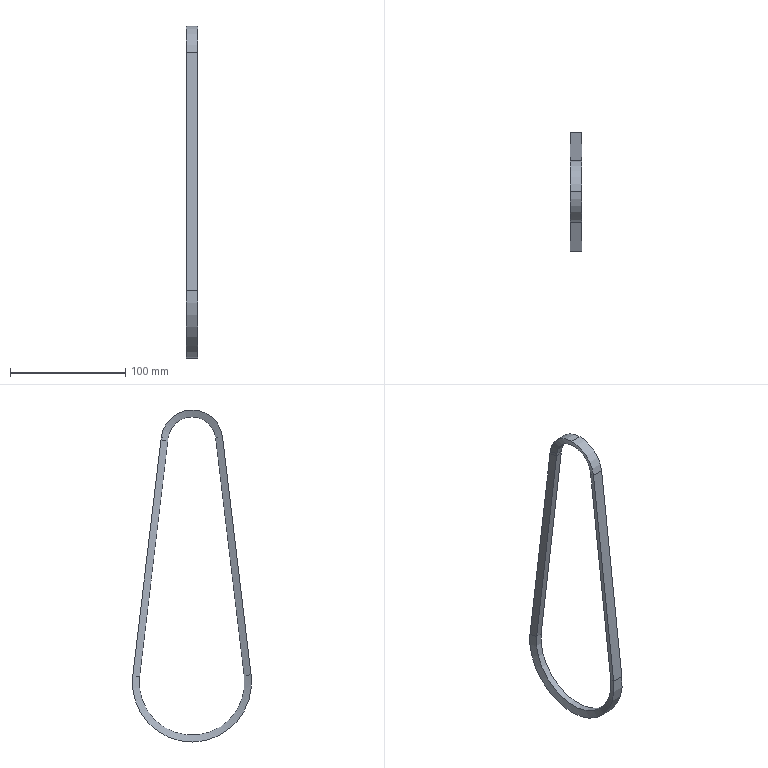Part | SolidWorks | features Sweep 1 | 1 solid | 22 faces | box 10 x 103.625 x 288.63 mm | volume 30426 mm3 | plane 12 | cylinder 6 | spline 4 | commonest cylinder face diameters 41.701 x2 53.634 x2 91.701 x1 103.625 x1
STEP:
#1=CARTESIAN_POINT('',(5.,-47.534,3.883));
#2=VERTEX_POINT('',#1);
#3=CARTESIAN_POINT('',(5.,-21.,26.817));
#4=VERTEX_POINT('',#3);
#5=CARTESIAN_POINT('',(5.,-21.,0.));
#6=DIRECTION('',(-1.,0.,0.));
#7=DIRECTION('',(0.,-0.9895,0.1448));
#8=AXIS2_PLACEMENT_3D('',#5,#6,#7);
#9=CIRCLE('',#8,26.817);
#10=EDGE_CURVE('',#2,#4,#9,.T.);
#11=ORIENTED_EDGE('',*,*,#10,.T.);
#12=CARTESIAN_POINT('',(-5.,-21.,26.817));
#13=VERTEX_POINT('',#12);
#14=CARTESIAN_POINT('',(0.,-21.,26.817));
#15=DIRECTION('',(-1.,0.,0.));
#16=VECTOR('',#15,1000.);
#17=LINE('',#14,#16);
#18=EDGE_CURVE('',#4,#13,#17,.T.);
#19=ORIENTED_EDGE('',*,*,#18,.T.);
#20=CARTESIAN_POINT('',(-5.,-47.534,3.883));
#21=VERTEX_POINT('',#20);
#22=CARTESIAN_POINT('',(-5.,-21.,0.));
#23=DIRECTION('',(-1.,0.,0.));
#24=DIRECTION('',(0.,-0.9895,0.1448));
#25=AXIS2_PLACEMENT_3D('',#22,#23,#24);
#26=CIRCLE('',#25,26.817);
#27=EDGE_CURVE('',#21,#13,#26,.T.);
#28=ORIENTED_EDGE('',*,*,#27,.F.);
#29=CARTESIAN_POINT('',(-5.,-47.534,3.883));
#30=DIRECTION('',(-1.,0.,0.));
#31=VECTOR('',#30,1000.);
#32=LINE('',#29,#31);
#33=EDGE_CURVE('',#2,#21,#32,.T.);
#34=ORIENTED_EDGE('',*,*,#33,.F.);
#35=EDGE_LOOP('',(#11,#19,#28,#34));
#36=FACE_OUTER_BOUND('',#35,.T.);
#37=CARTESIAN_POINT('',(0.,-21.,0.));
#38=DIRECTION('',(-1.,0.,0.));
#39=DIRECTION('',(0.,0.,1.));
#40=AXIS2_PLACEMENT_3D('',#37,#38,#39);
#41=CYLINDRICAL_SURFACE('',#40,26.817);
#42=ADVANCED_FACE('',(#36),#41,.T.);
#43=CARTESIAN_POINT('',(2.816,-21.,20.851));
#44=VERTEX_POINT('',#43);
#45=CARTESIAN_POINT('',(2.816,-0.2998,2.5));
#46=VERTEX_POINT('',#45);
#47=CARTESIAN_POINT('',(2.816,-21.,0.));
#48=DIRECTION('',(-1.,0.,0.));
#49=DIRECTION('',(0.,-0.993,0.1182));
#50=AXIS2_PLACEMENT_3D('',#47,#48,#49);
#51=CIRCLE('',#50,20.851);
#52=EDGE_CURVE('',#44,#46,#51,.T.);
#53=ORIENTED_EDGE('',*,*,#52,.F.);
#54=CARTESIAN_POINT('',(-2.816,-21.,20.851));
#55=VERTEX_POINT('',#54);
#56=CARTESIAN_POINT('',(0.,-21.,20.851));
#57=DIRECTION('',(-1.,0.,0.));
#58=VECTOR('',#57,1000.);
#59=LINE('',#56,#58);
#60=EDGE_CURVE('',#44,#55,#59,.T.);
#61=ORIENTED_EDGE('',*,*,#60,.T.);
#62=CARTESIAN_POINT('',(-2.816,-0.2998,2.5));
#63=VERTEX_POINT('',#62);
#64=CARTESIAN_POINT('',(-2.816,-21.,0.));
#65=DIRECTION('',(-1.,0.,0.));
#66=DIRECTION('',(0.,-0.993,0.1182));
#67=AXIS2_PLACEMENT_3D('',#64,#65,#66);
#68=CIRCLE('',#67,20.851);
#69=EDGE_CURVE('',#55,#63,#68,.T.);
#70=ORIENTED_EDGE('',*,*,#69,.T.);
#71=CARTESIAN_POINT('',(-2.816,-0.2998,2.5));
#72=DIRECTION('',(1.,0.,0.));
#73=VECTOR('',#72,1000.);
#74=LINE('',#71,#73);
#75=EDGE_CURVE('',#63,#46,#74,.T.);
#76=ORIENTED_EDGE('',*,*,#75,.T.);
#77=EDGE_LOOP('',(#53,#61,#70,#76));
#78=FACE_OUTER_BOUND('',#77,.T.);
#79=CARTESIAN_POINT('',(0.,-21.,0.));
#80=DIRECTION('',(-1.,0.,0.));
#81=DIRECTION('',(0.,0.,1.));
#82=AXIS2_PLACEMENT_3D('',#79,#80,#81);
#83=CYLINDRICAL_SURFACE('',#82,20.851);
#84=ADVANCED_FACE('',(#78),#83,.F.);
#85=CARTESIAN_POINT('',(-5.,5.7,2.5));
#86=VERTEX_POINT('',#85);
#87=CARTESIAN_POINT('',(-5.,5.7,2.5));
#88=DIRECTION('',(0.342,-0.9397,0.));
#89=VECTOR('',#88,1000.);
#90=LINE('',#87,#89);
#91=EDGE_CURVE('',#86,#63,#90,.T.);
#92=ORIENTED_EDGE('',*,*,#91,.F.);
#93=CARTESIAN_POINT('',(-5.,6.,0.));
#94=VERTEX_POINT('',#93);
#95=CARTESIAN_POINT('',(-5.,5.7,2.5));
#96=DIRECTION('',(0.,0.119,-0.9929));
#97=VECTOR('',#96,1000.);
#98=LINE('',#95,#97);
#99=EDGE_CURVE('',#86,#94,#98,.T.);
#100=ORIENTED_EDGE('',*,*,#99,.T.);
#101=CARTESIAN_POINT('',(-2.816,0.,0.));
#102=VERTEX_POINT('',#101);
#103=CARTESIAN_POINT('',(-5.,6.,0.));
#104=DIRECTION('',(0.342,-0.9397,0.));
#105=VECTOR('',#104,1000.);
#106=LINE('',#103,#105);
#107=EDGE_CURVE('',#94,#102,#106,.T.);
#108=ORIENTED_EDGE('',*,*,#107,.T.);
#109=CARTESIAN_POINT('',(-2.816,-0.2998,2.5));
#110=DIRECTION('',(0.,0.119,-0.9929));
#111=VECTOR('',#110,1000.);
#112=LINE('',#109,#111);
#113=EDGE_CURVE('',#63,#102,#112,.T.);
#114=ORIENTED_EDGE('',*,*,#113,.F.);
#115=EDGE_LOOP('',(#92,#100,#108,#114));
#116=FACE_OUTER_BOUND('',#115,.T.);
#117=CARTESIAN_POINT('',(-5.,5.7,2.5));
#118=DIRECTION('',(0.9389,0.3417,0.04097));
#119=DIRECTION('',(-0.342,0.9397,0.));
#120=AXIS2_PLACEMENT_3D('',#117,#118,#119);
#121=PLANE('',#120);
#122=ADVANCED_FACE('',(#116),#121,.F.);
#123=CARTESIAN_POINT('',(-2.816,24.522,-204.524));
#124=VERTEX_POINT('',#123);
#125=CARTESIAN_POINT('',(-2.816,0.,0.));
#126=DIRECTION('',(0.,0.119,-0.9929));
#127=VECTOR('',#126,1000.);
#128=LINE('',#125,#127);
#129=EDGE_CURVE('',#102,#124,#128,.T.);
#130=ORIENTED_EDGE('',*,*,#129,.F.);
#131=ORIENTED_EDGE('',*,*,#107,.F.);
#132=CARTESIAN_POINT('',(-5.,30.522,-204.524));
#133=VERTEX_POINT('',#132);
#134=CARTESIAN_POINT('',(-5.,6.,0.));
#135=DIRECTION('',(0.,0.119,-0.9929));
#136=VECTOR('',#135,1000.);
#137=LINE('',#134,#136);
#138=EDGE_CURVE('',#94,#133,#137,.T.);
#139=ORIENTED_EDGE('',*,*,#138,.T.);
#140=CARTESIAN_POINT('',(-5.,30.522,-204.524));
#141=DIRECTION('',(0.342,-0.9397,0.));
#142=VECTOR('',#141,1000.);
#143=LINE('',#140,#142);
#144=EDGE_CURVE('',#133,#124,#143,.T.);
#145=ORIENTED_EDGE('',*,*,#144,.T.);
#146=EDGE_LOOP('',(#130,#131,#139,#145));
#147=FACE_OUTER_BOUND('',#146,.T.);
#148=CARTESIAN_POINT('',(-5.,6.,0.));
#149=DIRECTION('',(0.9389,0.3417,0.04097));
#150=DIRECTION('',(-0.342,0.9397,0.));
#151=AXIS2_PLACEMENT_3D('',#148,#149,#150);
#152=PLANE('',#151);
#153=ADVANCED_FACE('',(#147),#152,.F.);
#154=CARTESIAN_POINT('',(2.816,0.,0.));
#155=VERTEX_POINT('',#154);
#156=CARTESIAN_POINT('',(2.816,24.522,-204.524));
#157=VERTEX_POINT('',#156);
#158=CARTESIAN_POINT('',(2.816,0.,0.));
#159=DIRECTION('',(0.,0.119,-0.9929));
#160=VECTOR('',#159,1000.);
#161=LINE('',#158,#160);
#162=EDGE_CURVE('',#155,#157,#161,.T.);
#163=ORIENTED_EDGE('',*,*,#162,.F.);
#164=CARTESIAN_POINT('',(-2.816,0.,0.));
#165=DIRECTION('',(1.,0.,0.));
#166=VECTOR('',#165,1000.);
#167=LINE('',#164,#166);
#168=EDGE_CURVE('',#102,#155,#167,.T.);
#169=ORIENTED_EDGE('',*,*,#168,.F.);
#170=ORIENTED_EDGE('',*,*,#129,.T.);
#171=CARTESIAN_POINT('',(-2.816,24.522,-204.524));
#172=DIRECTION('',(1.,0.,0.));
#173=VECTOR('',#172,1000.);
#174=LINE('',#171,#173);
#175=EDGE_CURVE('',#124,#157,#174,.T.);
#176=ORIENTED_EDGE('',*,*,#175,.T.);
#177=EDGE_LOOP('',(#163,#169,#170,#176));
#178=FACE_OUTER_BOUND('',#177,.T.);
#179=CARTESIAN_POINT('',(-2.816,0.,0.));
#180=DIRECTION('',(0.,0.9929,0.119));
#181=DIRECTION('',(0.,-0.119,0.9929));
#182=AXIS2_PLACEMENT_3D('',#179,#180,#181);
#183=PLANE('',#182);
#184=ADVANCED_FACE('',(#178),#183,.F.);
#185=CARTESIAN_POINT('',(5.,6.,0.));
#186=VERTEX_POINT('',#185);
#187=CARTESIAN_POINT('',(5.,30.522,-204.524));
#188=VERTEX_POINT('',#187);
#189=CARTESIAN_POINT('',(5.,6.,0.));
#190=DIRECTION('',(0.,0.119,-0.9929));
#191=VECTOR('',#190,1000.);
#192=LINE('',#189,#191);
#193=EDGE_CURVE('',#186,#188,#192,.T.);
#194=ORIENTED_EDGE('',*,*,#193,.F.);
#195=CARTESIAN_POINT('',(5.,6.,0.));
#196=DIRECTION('',(0.342,0.9397,0.));
#197=VECTOR('',#196,1000.);
#198=LINE('',#195,#197);
#199=EDGE_CURVE('',#155,#186,#198,.T.);
#200=ORIENTED_EDGE('',*,*,#199,.F.);
#201=ORIENTED_EDGE('',*,*,#162,.T.);
#202=CARTESIAN_POINT('',(5.,30.522,-204.524));
#203=DIRECTION('',(0.342,0.9397,0.));
#204=VECTOR('',#203,1000.);
#205=LINE('',#202,#204);
#206=EDGE_CURVE('',#157,#188,#205,.T.);
#207=ORIENTED_EDGE('',*,*,#206,.T.);
#208=EDGE_LOOP('',(#194,#200,#201,#207));
#209=FACE_OUTER_BOUND('',#208,.T.);
#210=CARTESIAN_POINT('',(5.,6.,0.));
#211=DIRECTION('',(-0.9389,0.3417,0.04097));
#212=DIRECTION('',(-0.342,-0.9397,0.));
#213=AXIS2_PLACEMENT_3D('',#210,#211,#212);
#214=PLANE('',#213);
#215=ADVANCED_FACE('',(#209),#214,.F.);
#216=CARTESIAN_POINT('',(-5.,30.522,-204.524));
#217=DIRECTION('',(-1.,0.,0.));
#218=VECTOR('',#217,1000.);
#219=LINE('',#216,#218);
#220=EDGE_CURVE('',#188,#133,#219,.T.);
#221=ORIENTED_EDGE('',*,*,#220,.T.);
#222=ORIENTED_EDGE('',*,*,#138,.F.);
#223=CARTESIAN_POINT('',(-5.,6.,0.));
#224=DIRECTION('',(-1.,0.,0.));
#225=VECTOR('',#224,1000.);
#226=LINE('',#223,#225);
#227=EDGE_CURVE('',#186,#94,#226,.T.);
#228=ORIENTED_EDGE('',*,*,#227,.F.);
#229=ORIENTED_EDGE('',*,*,#193,.T.);
#230=EDGE_LOOP('',(#221,#222,#228,#229));
#231=FACE_OUTER_BOUND('',#230,.T.);
#232=CARTESIAN_POINT('',(-5.,6.,0.));
#233=DIRECTION('',(0.,-0.9929,-0.119));
#234=DIRECTION('',(0.,0.119,-0.9929));
#235=AXIS2_PLACEMENT_3D('',#232,#233,#234);
#236=PLANE('',#235);
#237=ADVANCED_FACE('',(#231),#236,.F.);
#238=CARTESIAN_POINT('',(-2.816,-66.527,-204.559));
#239=VERTEX_POINT('',#238);
#240=CARTESIAN_POINT('',(-2.816,-21.,-210.));
#241=DIRECTION('',(-1.,0.,0.));
#242=DIRECTION('',(0.,0.9928,0.1194));
#243=AXIS2_PLACEMENT_3D('',#240,#241,#242);
#244=CIRCLE('',#243,45.851);
#245=EDGE_CURVE('',#124,#239,#244,.T.);
#246=ORIENTED_EDGE('',*,*,#245,.F.);
#247=ORIENTED_EDGE('',*,*,#144,.F.);
#248=CARTESIAN_POINT('',(-5.,-72.357,-203.141));
#249=VERTEX_POINT('',#248);
#250=CARTESIAN_POINT('',(-5.,-21.,-210.));
#251=DIRECTION('',(-1.,0.,0.));
#252=DIRECTION('',(0.,0.9944,0.1057));
#253=AXIS2_PLACEMENT_3D('',#250,#251,#252);
#254=CIRCLE('',#253,51.813);
#255=EDGE_CURVE('',#133,#249,#254,.T.);
#256=ORIENTED_EDGE('',*,*,#255,.T.);
#257=CARTESIAN_POINT('',(-5.,-72.357,-203.141));
#258=DIRECTION('',(0.342,0.9131,-0.2221));
#259=VECTOR('',#258,1000.);
#260=LINE('',#257,#259);
#261=EDGE_CURVE('',#249,#239,#260,.T.);
#262=ORIENTED_EDGE('',*,*,#261,.T.);
#263=EDGE_LOOP('',(#246,#247,#256,#262));
#264=FACE_OUTER_BOUND('',#263,.T.);
#265=CARTESIAN_POINT('',(-5.,30.522,-204.524));
#266=CARTESIAN_POINT('',(-5.,34.043,-237.642));
#267=CARTESIAN_POINT('',(-5.,11.606,-262.256));
#268=CARTESIAN_POINT('',(-5.,-21.696,-261.808));
#269=CARTESIAN_POINT('',(-5.,-54.998,-261.36));
#270=CARTESIAN_POINT('',(-5.,-76.766,-236.153));
#271=CARTESIAN_POINT('',(-5.,-72.357,-203.141));
#272=CARTESIAN_POINT('',(-2.816,24.522,-204.524));
#273=CARTESIAN_POINT('',(-2.816,28.043,-233.786));
#274=CARTESIAN_POINT('',(-2.816,8.491,-255.839));
#275=CARTESIAN_POINT('',(-2.816,-20.982,-255.851));
#276=CARTESIAN_POINT('',(-2.816,-50.455,-255.862));
#277=CARTESIAN_POINT('',(-2.816,-70.024,-233.824));
#278=CARTESIAN_POINT('',(-2.816,-66.527,-204.559));
#279=(BOUNDED_SURFACE()B_SPLINE_SURFACE(1,3,((#265,#266,#267,#268,#269,#270,#271),(#272,#273,#274,#275,#276,#277,#278)),.UNSPECIFIED.,.F.,.F.,.T.)B_SPLINE_SURFACE_WITH_KNOTS((2,2),(4,3,4),(0.,1.),(0.,0.5,1.),.UNSPECIFIED.)GEOMETRIC_REPRESENTATION_ITEM()RATIONAL_B_SPLINE_SURFACE(((1.,0.7758,0.7758,1.,0.7758,0.7758,1.),(1.,0.7758,0.7758,1.,0.7758,0.7758,1.)))REPRESENTATION_ITEM('')SURFACE());
#280=ADVANCED_FACE('',(#264),#279,.F.);
#281=CARTESIAN_POINT('',(2.816,-66.527,-204.559));
#282=VERTEX_POINT('',#281);
#283=CARTESIAN_POINT('',(2.816,-21.,-210.));
#284=DIRECTION('',(-1.,0.,0.));
#285=DIRECTION('',(0.,0.9928,0.1194));
#286=AXIS2_PLACEMENT_3D('',#283,#284,#285);
#287=CIRCLE('',#286,45.851);
#288=EDGE_CURVE('',#157,#282,#287,.T.);
#289=ORIENTED_EDGE('',*,*,#288,.F.);
#290=ORIENTED_EDGE('',*,*,#175,.F.);
#291=ORIENTED_EDGE('',*,*,#245,.T.);
#292=CARTESIAN_POINT('',(-2.816,-66.527,-204.559));
#293=DIRECTION('',(1.,0.,0.));
#294=VECTOR('',#293,1000.);
#295=LINE('',#292,#294);
#296=EDGE_CURVE('',#239,#282,#295,.T.);
#297=ORIENTED_EDGE('',*,*,#296,.T.);
#298=EDGE_LOOP('',(#289,#290,#291,#297));
#299=FACE_OUTER_BOUND('',#298,.T.);
#300=CARTESIAN_POINT('',(0.,-21.,-210.));
#301=DIRECTION('',(-1.,0.,0.));
#302=DIRECTION('',(0.,0.,1.));
#303=AXIS2_PLACEMENT_3D('',#300,#301,#302);
#304=CYLINDRICAL_SURFACE('',#303,45.851);
#305=ADVANCED_FACE('',(#299),#304,.F.);
#306=CARTESIAN_POINT('',(5.,-72.357,-203.141));
#307=VERTEX_POINT('',#306);
#308=CARTESIAN_POINT('',(5.,-21.,-210.));
#309=DIRECTION('',(-1.,0.,0.));
#310=DIRECTION('',(0.,0.9944,0.1057));
#311=AXIS2_PLACEMENT_3D('',#308,#309,#310);
#312=CIRCLE('',#311,51.813);
#313=EDGE_CURVE('',#188,#307,#312,.T.);
#314=ORIENTED_EDGE('',*,*,#313,.F.);
#315=ORIENTED_EDGE('',*,*,#206,.F.);
#316=ORIENTED_EDGE('',*,*,#288,.T.);
#317=CARTESIAN_POINT('',(5.,-72.357,-203.141));
#318=DIRECTION('',(0.342,-0.9131,0.2221));
#319=VECTOR('',#318,1000.);
#320=LINE('',#317,#319);
#321=EDGE_CURVE('',#282,#307,#320,.T.);
#322=ORIENTED_EDGE('',*,*,#321,.T.);
#323=EDGE_LOOP('',(#314,#315,#316,#322));
#324=FACE_OUTER_BOUND('',#323,.T.);
#325=CARTESIAN_POINT('',(2.816,24.522,-204.524));
#326=CARTESIAN_POINT('',(2.816,28.043,-233.786));
#327=CARTESIAN_POINT('',(2.816,8.491,-255.839));
#328=CARTESIAN_POINT('',(2.816,-20.982,-255.851));
#329=CARTESIAN_POINT('',(2.816,-50.455,-255.862));
#330=CARTESIAN_POINT('',(2.816,-70.024,-233.824));
#331=CARTESIAN_POINT('',(2.816,-66.527,-204.559));
#332=CARTESIAN_POINT('',(5.,30.522,-204.524));
#333=CARTESIAN_POINT('',(5.,34.043,-237.642));
#334=CARTESIAN_POINT('',(5.,11.606,-262.256));
#335=CARTESIAN_POINT('',(5.,-21.696,-261.808));
#336=CARTESIAN_POINT('',(5.,-54.998,-261.36));
#337=CARTESIAN_POINT('',(5.,-76.766,-236.153));
#338=CARTESIAN_POINT('',(5.,-72.357,-203.141));
#339=(BOUNDED_SURFACE()B_SPLINE_SURFACE(1,3,((#325,#326,#327,#328,#329,#330,#331),(#332,#333,#334,#335,#336,#337,#338)),.UNSPECIFIED.,.F.,.F.,.T.)B_SPLINE_SURFACE_WITH_KNOTS((2,2),(4,3,4),(0.,1.),(0.,0.5,1.),.UNSPECIFIED.)GEOMETRIC_REPRESENTATION_ITEM()RATIONAL_B_SPLINE_SURFACE(((1.,0.7758,0.7758,1.,0.7758,0.7758,1.),(1.,0.7758,0.7758,1.,0.7758,0.7758,1.)))REPRESENTATION_ITEM('')SURFACE());
#340=ADVANCED_FACE('',(#324),#339,.F.);
#341=CARTESIAN_POINT('',(-5.,-72.357,-203.141));
#342=DIRECTION('',(-1.,0.,0.));
#343=VECTOR('',#342,1000.);
#344=LINE('',#341,#343);
#345=EDGE_CURVE('',#307,#249,#344,.T.);
#346=ORIENTED_EDGE('',*,*,#345,.T.);
#347=ORIENTED_EDGE('',*,*,#255,.F.);
#348=ORIENTED_EDGE('',*,*,#220,.F.);
#349=ORIENTED_EDGE('',*,*,#313,.T.);
#350=EDGE_LOOP('',(#346,#347,#348,#349));
#351=FACE_OUTER_BOUND('',#350,.T.);
#352=CARTESIAN_POINT('',(0.,-21.,-210.));
#353=DIRECTION('',(-1.,0.,0.));
#354=DIRECTION('',(0.,0.,1.));
#355=AXIS2_PLACEMENT_3D('',#352,#353,#354);
#356=CYLINDRICAL_SURFACE('',#355,51.813);
#357=ADVANCED_FACE('',(#351),#356,.T.);
#358=CARTESIAN_POINT('',(-2.816,-41.705,2.464));
#359=VERTEX_POINT('',#358);
#360=CARTESIAN_POINT('',(-2.816,-66.527,-204.559));
#361=DIRECTION('',(0.,0.119,0.9929));
#362=VECTOR('',#361,1000.);
#363=LINE('',#360,#362);
#364=EDGE_CURVE('',#239,#359,#363,.T.);
#365=ORIENTED_EDGE('',*,*,#364,.F.);
#366=ORIENTED_EDGE('',*,*,#261,.F.);
#367=CARTESIAN_POINT('',(-5.,-72.357,-203.141));
#368=DIRECTION('',(0.,0.119,0.9929));
#369=VECTOR('',#368,1000.);
#370=LINE('',#367,#369);
#371=EDGE_CURVE('',#249,#21,#370,.T.);
#372=ORIENTED_EDGE('',*,*,#371,.T.);
#373=CARTESIAN_POINT('',(-5.,-47.534,3.883));
#374=DIRECTION('',(0.342,0.9131,-0.2221));
#375=VECTOR('',#374,1000.);
#376=LINE('',#373,#375);
#377=EDGE_CURVE('',#21,#359,#376,.T.);
#378=ORIENTED_EDGE('',*,*,#377,.T.);
#379=EDGE_LOOP('',(#365,#366,#372,#378));
#380=FACE_OUTER_BOUND('',#379,.T.);
#381=CARTESIAN_POINT('',(-5.,-72.357,-203.141));
#382=DIRECTION('',(0.9389,-0.3417,0.04097));
#383=DIRECTION('',(0.342,0.9397,0.));
#384=AXIS2_PLACEMENT_3D('',#381,#382,#383);
#385=PLANE('',#384);
#386=ADVANCED_FACE('',(#380),#385,.F.);
#387=CARTESIAN_POINT('',(2.816,-41.705,2.464));
#388=VERTEX_POINT('',#387);
#389=CARTESIAN_POINT('',(2.816,-66.527,-204.559));
#390=DIRECTION('',(0.,0.119,0.9929));
#391=VECTOR('',#390,1000.);
#392=LINE('',#389,#391);
#393=EDGE_CURVE('',#282,#388,#392,.T.);
#394=ORIENTED_EDGE('',*,*,#393,.F.);
#395=ORIENTED_EDGE('',*,*,#296,.F.);
#396=ORIENTED_EDGE('',*,*,#364,.T.);
#397=CARTESIAN_POINT('',(-2.816,-41.705,2.464));
#398=DIRECTION('',(1.,0.,0.));
#399=VECTOR('',#398,1000.);
#400=LINE('',#397,#399);
#401=EDGE_CURVE('',#359,#388,#400,.T.);
#402=ORIENTED_EDGE('',*,*,#401,.T.);
#403=EDGE_LOOP('',(#394,#395,#396,#402));
#404=FACE_OUTER_BOUND('',#403,.T.);
#405=CARTESIAN_POINT('',(-2.816,-66.527,-204.559));
#406=DIRECTION('',(0.,-0.9929,0.119));
#407=DIRECTION('',(0.,-0.119,-0.9929));
#408=AXIS2_PLACEMENT_3D('',#405,#406,#407);
#409=PLANE('',#408);
#410=ADVANCED_FACE('',(#404),#409,.F.);
#411=CARTESIAN_POINT('',(5.,-72.357,-203.141));
#412=DIRECTION('',(0.,0.119,0.9929));
#413=VECTOR('',#412,1000.);
#414=LINE('',#411,#413);
#415=EDGE_CURVE('',#307,#2,#414,.T.);
#416=ORIENTED_EDGE('',*,*,#415,.F.);
#417=ORIENTED_EDGE('',*,*,#321,.F.);
#418=ORIENTED_EDGE('',*,*,#393,.T.);
#419=CARTESIAN_POINT('',(5.,-47.534,3.883));
#420=DIRECTION('',(0.342,-0.9131,0.2221));
#421=VECTOR('',#420,1000.);
#422=LINE('',#419,#421);
#423=EDGE_CURVE('',#388,#2,#422,.T.);
#424=ORIENTED_EDGE('',*,*,#423,.T.);
#425=EDGE_LOOP('',(#416,#417,#418,#424));
#426=FACE_OUTER_BOUND('',#425,.T.);
#427=CARTESIAN_POINT('',(5.,-72.357,-203.141));
#428=DIRECTION('',(-0.9389,-0.3417,0.04097));
#429=DIRECTION('',(0.342,-0.9397,0.));
#430=AXIS2_PLACEMENT_3D('',#427,#428,#429);
#431=PLANE('',#430);
#432=ADVANCED_FACE('',(#426),#431,.F.);
#433=ORIENTED_EDGE('',*,*,#33,.T.);
#434=ORIENTED_EDGE('',*,*,#371,.F.);
#435=ORIENTED_EDGE('',*,*,#345,.F.);
#436=ORIENTED_EDGE('',*,*,#415,.T.);
#437=EDGE_LOOP('',(#433,#434,#435,#436));
#438=FACE_OUTER_BOUND('',#437,.T.);
#439=CARTESIAN_POINT('',(-5.,-72.357,-203.141));
#440=DIRECTION('',(0.,0.9929,-0.119));
#441=DIRECTION('',(0.,0.119,0.9929));
#442=AXIS2_PLACEMENT_3D('',#439,#440,#441);
#443=PLANE('',#442);
#444=ADVANCED_FACE('',(#438),#443,.F.);
#445=CARTESIAN_POINT('',(-2.816,-21.,0.));
#446=DIRECTION('',(-1.,0.,0.));
#447=DIRECTION('',(0.,-0.993,0.1182));
#448=AXIS2_PLACEMENT_3D('',#445,#446,#447);
#449=CIRCLE('',#448,20.851);
#450=EDGE_CURVE('',#359,#55,#449,.T.);
#451=ORIENTED_EDGE('',*,*,#450,.F.);
#452=ORIENTED_EDGE('',*,*,#377,.F.);
#453=ORIENTED_EDGE('',*,*,#27,.T.);
#454=CARTESIAN_POINT('',(-5.,-21.,0.));
#455=DIRECTION('',(-1.,0.,0.));
#456=DIRECTION('',(0.,-0.9895,0.1448));
#457=AXIS2_PLACEMENT_3D('',#454,#455,#456);
#458=CIRCLE('',#457,26.817);
#459=EDGE_CURVE('',#13,#86,#458,.T.);
#460=ORIENTED_EDGE('',*,*,#459,.T.);
#461=ORIENTED_EDGE('',*,*,#91,.T.);
#462=ORIENTED_EDGE('',*,*,#69,.F.);
#463=EDGE_LOOP('',(#451,#452,#453,#460,#461,#462));
#464=FACE_OUTER_BOUND('',#463,.T.);
#465=CARTESIAN_POINT('',(-5.,-47.534,3.883));
#466=CARTESIAN_POINT('',(-5.,-41.307,46.441));
#467=CARTESIAN_POINT('',(-5.,1.691,45.324));
#468=CARTESIAN_POINT('',(-5.,5.7,2.5));
#469=CARTESIAN_POINT('',(-2.816,-41.705,2.464));
#470=CARTESIAN_POINT('',(-2.816,-37.752,35.672));
#471=CARTESIAN_POINT('',(-2.816,-4.309,35.701));
#472=CARTESIAN_POINT('',(-2.816,-0.2998,2.5));
#473=(BOUNDED_SURFACE()B_SPLINE_SURFACE(1,3,((#465,#466,#467,#468),(#469,#470,#471,#472)),.UNSPECIFIED.,.F.,.F.,.F.)B_SPLINE_SURFACE_WITH_KNOTS((2,2),(4,4),(0.,1.),(0.,1.),.UNSPECIFIED.)GEOMETRIC_REPRESENTATION_ITEM()RATIONAL_B_SPLINE_SURFACE(((1.,0.4127,0.4127,1.),(1.,0.4127,0.4127,1.)))REPRESENTATION_ITEM('')SURFACE());
#474=ADVANCED_FACE('',(#464),#473,.F.);
#475=ORIENTED_EDGE('',*,*,#60,.F.);
#476=CARTESIAN_POINT('',(2.816,-21.,0.));
#477=DIRECTION('',(-1.,0.,0.));
#478=DIRECTION('',(0.,-0.993,0.1182));
#479=AXIS2_PLACEMENT_3D('',#476,#477,#478);
#480=CIRCLE('',#479,20.851);
#481=EDGE_CURVE('',#388,#44,#480,.T.);
#482=ORIENTED_EDGE('',*,*,#481,.F.);
#483=ORIENTED_EDGE('',*,*,#401,.F.);
#484=ORIENTED_EDGE('',*,*,#450,.T.);
#485=EDGE_LOOP('',(#475,#482,#483,#484));
#486=FACE_OUTER_BOUND('',#485,.T.);
#487=CARTESIAN_POINT('',(0.,-21.,0.));
#488=DIRECTION('',(-1.,0.,0.));
#489=DIRECTION('',(0.,0.,1.));
#490=AXIS2_PLACEMENT_3D('',#487,#488,#489);
#491=CYLINDRICAL_SURFACE('',#490,20.851);
#492=ADVANCED_FACE('',(#486),#491,.F.);
#493=ORIENTED_EDGE('',*,*,#10,.F.);
#494=ORIENTED_EDGE('',*,*,#423,.F.);
#495=ORIENTED_EDGE('',*,*,#481,.T.);
#496=ORIENTED_EDGE('',*,*,#52,.T.);
#497=CARTESIAN_POINT('',(5.,5.7,2.5));
#498=VERTEX_POINT('',#497);
#499=CARTESIAN_POINT('',(5.,5.7,2.5));
#500=DIRECTION('',(0.342,0.9397,0.));
#501=VECTOR('',#500,1000.);
#502=LINE('',#499,#501);
#503=EDGE_CURVE('',#46,#498,#502,.T.);
#504=ORIENTED_EDGE('',*,*,#503,.T.);
#505=CARTESIAN_POINT('',(5.,-21.,0.));
#506=DIRECTION('',(-1.,0.,0.));
#507=DIRECTION('',(0.,-0.9895,0.1448));
#508=AXIS2_PLACEMENT_3D('',#505,#506,#507);
#509=CIRCLE('',#508,26.817);
#510=EDGE_CURVE('',#4,#498,#509,.T.);
#511=ORIENTED_EDGE('',*,*,#510,.F.);
#512=EDGE_LOOP('',(#493,#494,#495,#496,#504,#511));
#513=FACE_OUTER_BOUND('',#512,.T.);
#514=CARTESIAN_POINT('',(2.816,-41.705,2.464));
#515=CARTESIAN_POINT('',(2.816,-37.752,35.672));
#516=CARTESIAN_POINT('',(2.816,-4.309,35.701));
#517=CARTESIAN_POINT('',(2.816,-0.2998,2.5));
#518=CARTESIAN_POINT('',(5.,-47.534,3.883));
#519=CARTESIAN_POINT('',(5.,-41.307,46.441));
#520=CARTESIAN_POINT('',(5.,1.691,45.324));
#521=CARTESIAN_POINT('',(5.,5.7,2.5));
#522=(BOUNDED_SURFACE()B_SPLINE_SURFACE(1,3,((#514,#515,#516,#517),(#518,#519,#520,#521)),.UNSPECIFIED.,.F.,.F.,.F.)B_SPLINE_SURFACE_WITH_KNOTS((2,2),(4,4),(0.,1.),(0.,1.),.UNSPECIFIED.)GEOMETRIC_REPRESENTATION_ITEM()RATIONAL_B_SPLINE_SURFACE(((1.,0.4127,0.4127,1.),(1.,0.4127,0.4127,1.)))REPRESENTATION_ITEM('')SURFACE());
#523=ADVANCED_FACE('',(#513),#522,.F.);
#524=ORIENTED_EDGE('',*,*,#18,.F.);
#525=ORIENTED_EDGE('',*,*,#510,.T.);
#526=CARTESIAN_POINT('',(-5.,5.7,2.5));
#527=DIRECTION('',(-1.,0.,0.));
#528=VECTOR('',#527,1000.);
#529=LINE('',#526,#528);
#530=EDGE_CURVE('',#498,#86,#529,.T.);
#531=ORIENTED_EDGE('',*,*,#530,.T.);
#532=ORIENTED_EDGE('',*,*,#459,.F.);
#533=EDGE_LOOP('',(#524,#525,#531,#532));
#534=FACE_OUTER_BOUND('',#533,.T.);
#535=CARTESIAN_POINT('',(0.,-21.,0.));
#536=DIRECTION('',(-1.,0.,0.));
#537=DIRECTION('',(0.,0.,1.));
#538=AXIS2_PLACEMENT_3D('',#535,#536,#537);
#539=CYLINDRICAL_SURFACE('',#538,26.817);
#540=ADVANCED_FACE('',(#534),#539,.T.);
#541=ORIENTED_EDGE('',*,*,#113,.T.);
#542=ORIENTED_EDGE('',*,*,#168,.T.);
#543=CARTESIAN_POINT('',(2.816,-0.2998,2.5));
#544=DIRECTION('',(0.,0.119,-0.9929));
#545=VECTOR('',#544,1000.);
#546=LINE('',#543,#545);
#547=EDGE_CURVE('',#46,#155,#546,.T.);
#548=ORIENTED_EDGE('',*,*,#547,.F.);
#549=ORIENTED_EDGE('',*,*,#75,.F.);
#550=EDGE_LOOP('',(#541,#542,#548,#549));
#551=FACE_OUTER_BOUND('',#550,.T.);
#552=CARTESIAN_POINT('',(-2.816,-0.2998,2.5));
#553=DIRECTION('',(0.,0.9929,0.119));
#554=DIRECTION('',(0.,-0.119,0.9929));
#555=AXIS2_PLACEMENT_3D('',#552,#553,#554);
#556=PLANE('',#555);
#557=ADVANCED_FACE('',(#551),#556,.F.);
#558=ORIENTED_EDGE('',*,*,#547,.T.);
#559=ORIENTED_EDGE('',*,*,#199,.T.);
#560=CARTESIAN_POINT('',(5.,5.7,2.5));
#561=DIRECTION('',(0.,0.119,-0.9929));
#562=VECTOR('',#561,1000.);
#563=LINE('',#560,#562);
#564=EDGE_CURVE('',#498,#186,#563,.T.);
#565=ORIENTED_EDGE('',*,*,#564,.F.);
#566=ORIENTED_EDGE('',*,*,#503,.F.);
#567=EDGE_LOOP('',(#558,#559,#565,#566));
#568=FACE_OUTER_BOUND('',#567,.T.);
#569=CARTESIAN_POINT('',(5.,5.7,2.5));
#570=DIRECTION('',(-0.9389,0.3417,0.04097));
#571=DIRECTION('',(-0.342,-0.9397,0.));
#572=AXIS2_PLACEMENT_3D('',#569,#570,#571);
#573=PLANE('',#572);
#574=ADVANCED_FACE('',(#568),#573,.F.);
#575=ORIENTED_EDGE('',*,*,#564,.T.);
#576=ORIENTED_EDGE('',*,*,#227,.T.);
#577=ORIENTED_EDGE('',*,*,#99,.F.);
#578=ORIENTED_EDGE('',*,*,#530,.F.);
#579=EDGE_LOOP('',(#575,#576,#577,#578));
#580=FACE_OUTER_BOUND('',#579,.T.);
#581=CARTESIAN_POINT('',(-5.,5.7,2.5));
#582=DIRECTION('',(0.,-0.9929,-0.119));
#583=DIRECTION('',(0.,0.119,-0.9929));
#584=AXIS2_PLACEMENT_3D('',#581,#582,#583);
#585=PLANE('',#584);
#586=ADVANCED_FACE('',(#580),#585,.F.);
#587=CLOSED_SHELL('',(#42,#84,#122,#153,#184,#215,#237,#280,#305,#340,#357,#386,#410,#432,#444,#474,#492,#523,#540,#557,#574,#586));
#588=MANIFOLD_SOLID_BREP('',#587);
#589=CARTESIAN_POINT('',(0.,0.,0.));
#590=DIRECTION('',(0.,0.,1.));
#591=DIRECTION('',(1.,0.,0.));
#592=AXIS2_PLACEMENT_3D('',#589,#590,#591);
#593=(LENGTH_UNIT()NAMED_UNIT(*)SI_UNIT(.MILLI.,.METRE.));
#594=UNCERTAINTY_MEASURE_WITH_UNIT(LENGTH_MEASURE(0.00001),#593,'','');
#595=(NAMED_UNIT(*)PLANE_ANGLE_UNIT()SI_UNIT($,.RADIAN.));
#596=(NAMED_UNIT(*)SI_UNIT($,.STERADIAN.)SOLID_ANGLE_UNIT());
#597=(GEOMETRIC_REPRESENTATION_CONTEXT(3)GLOBAL_UNCERTAINTY_ASSIGNED_CONTEXT((#594))GLOBAL_UNIT_ASSIGNED_CONTEXT((#593,#595,#596))REPRESENTATION_CONTEXT('',''));
#598=ADVANCED_BREP_SHAPE_REPRESENTATION('',(#588,#592),#597);